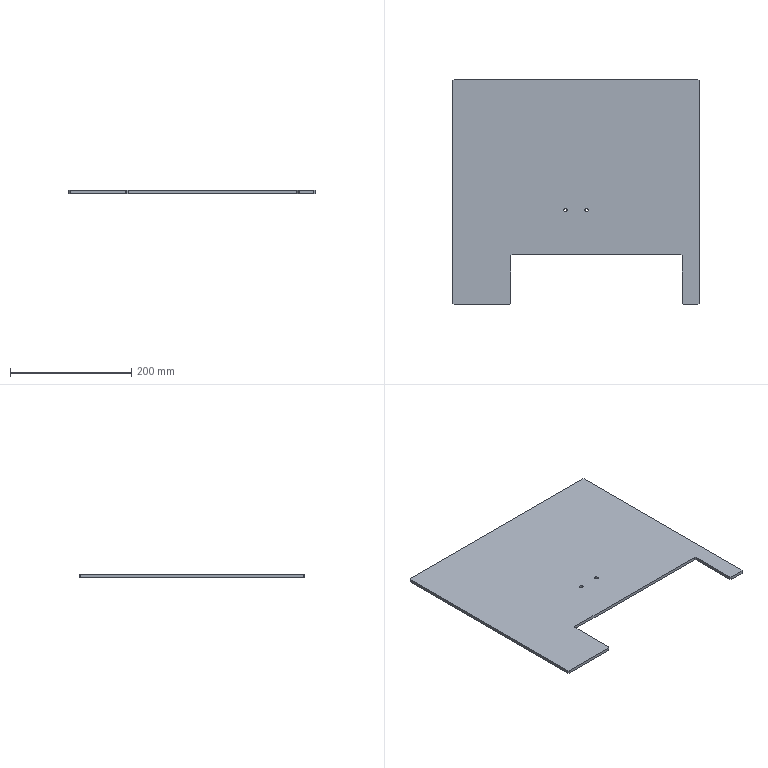Part | SolidWorks | features Extrusion 1, Fillet 1, HoleWzd 1, ICE 1 | 1 solid | 22 faces | box 406 x 372 x 5 mm | volume 637645 mm3 | plane 18 | cylinder 4 | commonest cylinder face diameters 5.5 x4
STEP:
#1=CARTESIAN_POINT('',(-20.25,-30.,0.));
#2=VERTEX_POINT('',#1);
#3=CARTESIAN_POINT('',(-14.75,-30.,0.));
#4=VERTEX_POINT('',#3);
#5=CARTESIAN_POINT('',(-17.5,-30.,0.));
#6=DIRECTION('',(0.,0.,1.));
#7=DIRECTION('',(1.,0.,0.));
#8=AXIS2_PLACEMENT_3D('',#5,#6,#7);
#9=CIRCLE('',#8,2.75);
#10=EDGE_CURVE('',#2,#4,#9,.T.);
#11=ORIENTED_EDGE('',*,*,#10,.F.);
#12=CARTESIAN_POINT('',(-20.25,-30.,5.));
#13=VERTEX_POINT('',#12);
#14=CARTESIAN_POINT('',(-20.25,-30.,5.));
#15=DIRECTION('',(0.,0.,1.));
#16=VECTOR('',#15,1000.);
#17=LINE('',#14,#16);
#18=EDGE_CURVE('',#2,#13,#17,.T.);
#19=ORIENTED_EDGE('',*,*,#18,.T.);
#20=CARTESIAN_POINT('',(-14.75,-30.,5.));
#21=VERTEX_POINT('',#20);
#22=CARTESIAN_POINT('',(-17.5,-30.,5.));
#23=DIRECTION('',(0.,0.,1.));
#24=DIRECTION('',(1.,0.,0.));
#25=AXIS2_PLACEMENT_3D('',#22,#23,#24);
#26=CIRCLE('',#25,2.75);
#27=EDGE_CURVE('',#13,#21,#26,.T.);
#28=ORIENTED_EDGE('',*,*,#27,.T.);
#29=CARTESIAN_POINT('',(-14.75,-30.,5.));
#30=DIRECTION('',(0.,0.,1.));
#31=VECTOR('',#30,1000.);
#32=LINE('',#29,#31);
#33=EDGE_CURVE('',#4,#21,#32,.T.);
#34=ORIENTED_EDGE('',*,*,#33,.F.);
#35=EDGE_LOOP('',(#11,#19,#28,#34));
#36=FACE_OUTER_BOUND('',#35,.T.);
#37=CARTESIAN_POINT('',(-17.5,-30.,5.));
#38=DIRECTION('',(0.,0.,1.));
#39=DIRECTION('',(1.,0.,0.));
#40=AXIS2_PLACEMENT_3D('',#37,#38,#39);
#41=CYLINDRICAL_SURFACE('',#40,2.75);
#42=ADVANCED_FACE('',(#36),#41,.F.);
#43=CARTESIAN_POINT('',(14.75,-30.,0.));
#44=VERTEX_POINT('',#43);
#45=CARTESIAN_POINT('',(20.25,-30.,0.));
#46=VERTEX_POINT('',#45);
#47=CARTESIAN_POINT('',(17.5,-30.,0.));
#48=DIRECTION('',(0.,0.,1.));
#49=DIRECTION('',(1.,0.,0.));
#50=AXIS2_PLACEMENT_3D('',#47,#48,#49);
#51=CIRCLE('',#50,2.75);
#52=EDGE_CURVE('',#44,#46,#51,.T.);
#53=ORIENTED_EDGE('',*,*,#52,.F.);
#54=CARTESIAN_POINT('',(14.75,-30.,5.));
#55=VERTEX_POINT('',#54);
#56=CARTESIAN_POINT('',(14.75,-30.,5.));
#57=DIRECTION('',(0.,0.,1.));
#58=VECTOR('',#57,1000.);
#59=LINE('',#56,#58);
#60=EDGE_CURVE('',#44,#55,#59,.T.);
#61=ORIENTED_EDGE('',*,*,#60,.T.);
#62=CARTESIAN_POINT('',(20.25,-30.,5.));
#63=VERTEX_POINT('',#62);
#64=CARTESIAN_POINT('',(17.5,-30.,5.));
#65=DIRECTION('',(0.,0.,1.));
#66=DIRECTION('',(1.,0.,0.));
#67=AXIS2_PLACEMENT_3D('',#64,#65,#66);
#68=CIRCLE('',#67,2.75);
#69=EDGE_CURVE('',#55,#63,#68,.T.);
#70=ORIENTED_EDGE('',*,*,#69,.T.);
#71=CARTESIAN_POINT('',(20.25,-30.,5.));
#72=DIRECTION('',(0.,0.,1.));
#73=VECTOR('',#72,1000.);
#74=LINE('',#71,#73);
#75=EDGE_CURVE('',#46,#63,#74,.T.);
#76=ORIENTED_EDGE('',*,*,#75,.F.);
#77=EDGE_LOOP('',(#53,#61,#70,#76));
#78=FACE_OUTER_BOUND('',#77,.T.);
#79=CARTESIAN_POINT('',(17.5,-30.,5.));
#80=DIRECTION('',(0.,0.,1.));
#81=DIRECTION('',(1.,0.,0.));
#82=AXIS2_PLACEMENT_3D('',#79,#80,#81);
#83=CYLINDRICAL_SURFACE('',#82,2.75);
#84=ADVANCED_FACE('',(#78),#83,.F.);
#85=CARTESIAN_POINT('',(-201.,-186.,0.));
#86=VERTEX_POINT('',#85);
#87=CARTESIAN_POINT('',(-109.5,-186.,0.));
#88=VERTEX_POINT('',#87);
#89=CARTESIAN_POINT('',(203.,-186.,0.));
#90=DIRECTION('',(1.,0.,0.));
#91=VECTOR('',#90,1000.);
#92=LINE('',#89,#91);
#93=EDGE_CURVE('',#86,#88,#92,.T.);
#94=ORIENTED_EDGE('',*,*,#93,.T.);
#95=CARTESIAN_POINT('',(-109.5,-186.,5.));
#96=VERTEX_POINT('',#95);
#97=CARTESIAN_POINT('',(-109.5,-186.,5.));
#98=DIRECTION('',(0.,0.,1.));
#99=VECTOR('',#98,1000.);
#100=LINE('',#97,#99);
#101=EDGE_CURVE('',#88,#96,#100,.T.);
#102=ORIENTED_EDGE('',*,*,#101,.T.);
#103=CARTESIAN_POINT('',(-201.,-186.,5.));
#104=VERTEX_POINT('',#103);
#105=CARTESIAN_POINT('',(203.,-186.,5.));
#106=DIRECTION('',(1.,0.,0.));
#107=VECTOR('',#106,1000.);
#108=LINE('',#105,#107);
#109=EDGE_CURVE('',#104,#96,#108,.T.);
#110=ORIENTED_EDGE('',*,*,#109,.F.);
#111=CARTESIAN_POINT('',(-201.,-186.,5.));
#112=DIRECTION('',(0.,0.,-1.));
#113=VECTOR('',#112,1000.);
#114=LINE('',#111,#113);
#115=EDGE_CURVE('',#104,#86,#114,.T.);
#116=ORIENTED_EDGE('',*,*,#115,.T.);
#117=EDGE_LOOP('',(#94,#102,#110,#116));
#118=FACE_OUTER_BOUND('',#117,.T.);
#119=CARTESIAN_POINT('',(203.,-186.,5.));
#120=DIRECTION('',(0.,1.,0.));
#121=DIRECTION('',(-1.,0.,0.));
#122=AXIS2_PLACEMENT_3D('',#119,#120,#121);
#123=PLANE('',#122);
#124=ADVANCED_FACE('',(#118),#123,.F.);
#125=CARTESIAN_POINT('',(-203.,184.,5.));
#126=VERTEX_POINT('',#125);
#127=CARTESIAN_POINT('',(-203.,-184.,5.));
#128=VERTEX_POINT('',#127);
#129=CARTESIAN_POINT('',(-203.,-186.,5.));
#130=DIRECTION('',(0.,-1.,0.));
#131=VECTOR('',#130,1000.);
#132=LINE('',#129,#131);
#133=EDGE_CURVE('',#126,#128,#132,.T.);
#134=ORIENTED_EDGE('',*,*,#133,.F.);
#135=CARTESIAN_POINT('',(-203.,184.,0.));
#136=VERTEX_POINT('',#135);
#137=CARTESIAN_POINT('',(-203.,184.,5.));
#138=DIRECTION('',(0.,0.,-1.));
#139=VECTOR('',#138,1000.);
#140=LINE('',#137,#139);
#141=EDGE_CURVE('',#126,#136,#140,.T.);
#142=ORIENTED_EDGE('',*,*,#141,.T.);
#143=CARTESIAN_POINT('',(-203.,-184.,0.));
#144=VERTEX_POINT('',#143);
#145=CARTESIAN_POINT('',(-203.,-186.,0.));
#146=DIRECTION('',(0.,-1.,0.));
#147=VECTOR('',#146,1000.);
#148=LINE('',#145,#147);
#149=EDGE_CURVE('',#136,#144,#148,.T.);
#150=ORIENTED_EDGE('',*,*,#149,.T.);
#151=CARTESIAN_POINT('',(-203.,-184.,5.));
#152=DIRECTION('',(0.,0.,1.));
#153=VECTOR('',#152,1000.);
#154=LINE('',#151,#153);
#155=EDGE_CURVE('',#144,#128,#154,.T.);
#156=ORIENTED_EDGE('',*,*,#155,.T.);
#157=EDGE_LOOP('',(#134,#142,#150,#156));
#158=FACE_OUTER_BOUND('',#157,.T.);
#159=CARTESIAN_POINT('',(-203.,-186.,5.));
#160=DIRECTION('',(1.,0.,0.));
#161=DIRECTION('',(0.,0.,-1.));
#162=AXIS2_PLACEMENT_3D('',#159,#160,#161);
#163=PLANE('',#162);
#164=ADVANCED_FACE('',(#158),#163,.F.);
#165=CARTESIAN_POINT('',(177.,-186.,5.));
#166=VERTEX_POINT('',#165);
#167=CARTESIAN_POINT('',(201.,-186.,5.));
#168=VERTEX_POINT('',#167);
#169=CARTESIAN_POINT('',(203.,-186.,5.));
#170=DIRECTION('',(1.,0.,0.));
#171=VECTOR('',#170,1000.);
#172=LINE('',#169,#171);
#173=EDGE_CURVE('',#166,#168,#172,.T.);
#174=ORIENTED_EDGE('',*,*,#173,.F.);
#175=CARTESIAN_POINT('',(177.,-186.,0.));
#176=VERTEX_POINT('',#175);
#177=CARTESIAN_POINT('',(177.,-186.,5.));
#178=DIRECTION('',(0.,0.,-1.));
#179=VECTOR('',#178,1000.);
#180=LINE('',#177,#179);
#181=EDGE_CURVE('',#166,#176,#180,.T.);
#182=ORIENTED_EDGE('',*,*,#181,.T.);
#183=CARTESIAN_POINT('',(201.,-186.,0.));
#184=VERTEX_POINT('',#183);
#185=CARTESIAN_POINT('',(203.,-186.,0.));
#186=DIRECTION('',(1.,0.,0.));
#187=VECTOR('',#186,1000.);
#188=LINE('',#185,#187);
#189=EDGE_CURVE('',#176,#184,#188,.T.);
#190=ORIENTED_EDGE('',*,*,#189,.T.);
#191=CARTESIAN_POINT('',(201.,-186.,5.));
#192=DIRECTION('',(0.,0.,1.));
#193=VECTOR('',#192,1000.);
#194=LINE('',#191,#193);
#195=EDGE_CURVE('',#184,#168,#194,.T.);
#196=ORIENTED_EDGE('',*,*,#195,.T.);
#197=EDGE_LOOP('',(#174,#182,#190,#196));
#198=FACE_OUTER_BOUND('',#197,.T.);
#199=CARTESIAN_POINT('',(203.,-186.,5.));
#200=DIRECTION('',(0.,1.,0.));
#201=DIRECTION('',(-1.,0.,0.));
#202=AXIS2_PLACEMENT_3D('',#199,#200,#201);
#203=PLANE('',#202);
#204=ADVANCED_FACE('',(#198),#203,.F.);
#205=CARTESIAN_POINT('',(203.,-184.,0.));
#206=VERTEX_POINT('',#205);
#207=CARTESIAN_POINT('',(203.,184.,0.));
#208=VERTEX_POINT('',#207);
#209=CARTESIAN_POINT('',(203.,-186.,0.));
#210=DIRECTION('',(0.,1.,0.));
#211=VECTOR('',#210,1000.);
#212=LINE('',#209,#211);
#213=EDGE_CURVE('',#206,#208,#212,.T.);
#214=ORIENTED_EDGE('',*,*,#213,.T.);
#215=CARTESIAN_POINT('',(203.,184.,5.));
#216=VERTEX_POINT('',#215);
#217=CARTESIAN_POINT('',(203.,184.,5.));
#218=DIRECTION('',(0.,0.,1.));
#219=VECTOR('',#218,1000.);
#220=LINE('',#217,#219);
#221=EDGE_CURVE('',#208,#216,#220,.T.);
#222=ORIENTED_EDGE('',*,*,#221,.T.);
#223=CARTESIAN_POINT('',(203.,-184.,5.));
#224=VERTEX_POINT('',#223);
#225=CARTESIAN_POINT('',(203.,-186.,5.));
#226=DIRECTION('',(0.,1.,0.));
#227=VECTOR('',#226,1000.);
#228=LINE('',#225,#227);
#229=EDGE_CURVE('',#224,#216,#228,.T.);
#230=ORIENTED_EDGE('',*,*,#229,.F.);
#231=CARTESIAN_POINT('',(203.,-184.,5.));
#232=DIRECTION('',(0.,0.,-1.));
#233=VECTOR('',#232,1000.);
#234=LINE('',#231,#233);
#235=EDGE_CURVE('',#224,#206,#234,.T.);
#236=ORIENTED_EDGE('',*,*,#235,.T.);
#237=EDGE_LOOP('',(#214,#222,#230,#236));
#238=FACE_OUTER_BOUND('',#237,.T.);
#239=CARTESIAN_POINT('',(203.,-186.,5.));
#240=DIRECTION('',(-1.,0.,0.));
#241=DIRECTION('',(0.,-1.,0.));
#242=AXIS2_PLACEMENT_3D('',#239,#240,#241);
#243=PLANE('',#242);
#244=ADVANCED_FACE('',(#238),#243,.F.);
#245=CARTESIAN_POINT('',(201.,186.,0.));
#246=VERTEX_POINT('',#245);
#247=CARTESIAN_POINT('',(-201.,186.,0.));
#248=VERTEX_POINT('',#247);
#249=CARTESIAN_POINT('',(203.,186.,0.));
#250=DIRECTION('',(-1.,0.,0.));
#251=VECTOR('',#250,1000.);
#252=LINE('',#249,#251);
#253=EDGE_CURVE('',#246,#248,#252,.T.);
#254=ORIENTED_EDGE('',*,*,#253,.T.);
#255=CARTESIAN_POINT('',(-201.,186.,5.));
#256=VERTEX_POINT('',#255);
#257=CARTESIAN_POINT('',(-201.,186.,5.));
#258=DIRECTION('',(0.,0.,1.));
#259=VECTOR('',#258,1000.);
#260=LINE('',#257,#259);
#261=EDGE_CURVE('',#248,#256,#260,.T.);
#262=ORIENTED_EDGE('',*,*,#261,.T.);
#263=CARTESIAN_POINT('',(201.,186.,5.));
#264=VERTEX_POINT('',#263);
#265=CARTESIAN_POINT('',(203.,186.,5.));
#266=DIRECTION('',(-1.,0.,0.));
#267=VECTOR('',#266,1000.);
#268=LINE('',#265,#267);
#269=EDGE_CURVE('',#264,#256,#268,.T.);
#270=ORIENTED_EDGE('',*,*,#269,.F.);
#271=CARTESIAN_POINT('',(201.,186.,5.));
#272=DIRECTION('',(0.,0.,-1.));
#273=VECTOR('',#272,1000.);
#274=LINE('',#271,#273);
#275=EDGE_CURVE('',#264,#246,#274,.T.);
#276=ORIENTED_EDGE('',*,*,#275,.T.);
#277=EDGE_LOOP('',(#254,#262,#270,#276));
#278=FACE_OUTER_BOUND('',#277,.T.);
#279=CARTESIAN_POINT('',(203.,186.,5.));
#280=DIRECTION('',(0.,-1.,0.));
#281=DIRECTION('',(1.,0.,0.));
#282=AXIS2_PLACEMENT_3D('',#279,#280,#281);
#283=PLANE('',#282);
#284=ADVANCED_FACE('',(#278),#283,.F.);
#285=CARTESIAN_POINT('',(-17.5,-30.,5.));
#286=DIRECTION('',(0.,0.,1.));
#287=DIRECTION('',(1.,0.,0.));
#288=AXIS2_PLACEMENT_3D('',#285,#286,#287);
#289=CIRCLE('',#288,2.75);
#290=EDGE_CURVE('',#21,#13,#289,.T.);
#291=ORIENTED_EDGE('',*,*,#290,.F.);
#292=ORIENTED_EDGE('',*,*,#27,.F.);
#293=EDGE_LOOP('',(#291,#292));
#294=FACE_BOUND('',#293,.T.);
#295=CARTESIAN_POINT('',(17.5,-30.,5.));
#296=DIRECTION('',(0.,0.,1.));
#297=DIRECTION('',(1.,0.,0.));
#298=AXIS2_PLACEMENT_3D('',#295,#296,#297);
#299=CIRCLE('',#298,2.75);
#300=EDGE_CURVE('',#63,#55,#299,.T.);
#301=ORIENTED_EDGE('',*,*,#300,.F.);
#302=ORIENTED_EDGE('',*,*,#69,.F.);
#303=EDGE_LOOP('',(#301,#302));
#304=FACE_BOUND('',#303,.T.);
#305=CARTESIAN_POINT('',(175.,-184.,5.));
#306=VERTEX_POINT('',#305);
#307=CARTESIAN_POINT('',(175.,-105.,5.));
#308=VERTEX_POINT('',#307);
#309=CARTESIAN_POINT('',(175.,-186.,5.));
#310=DIRECTION('',(0.,1.,0.));
#311=VECTOR('',#310,1000.);
#312=LINE('',#309,#311);
#313=EDGE_CURVE('',#306,#308,#312,.T.);
#314=ORIENTED_EDGE('',*,*,#313,.F.);
#315=CARTESIAN_POINT('',(-4.5,-4.5,5.));
#316=DIRECTION('',(0.7071,-0.7071,0.));
#317=VECTOR('',#316,1000.);
#318=LINE('',#315,#317);
#319=EDGE_CURVE('',#306,#166,#318,.T.);
#320=ORIENTED_EDGE('',*,*,#319,.T.);
#321=ORIENTED_EDGE('',*,*,#173,.T.);
#322=CARTESIAN_POINT('',(193.5,-193.5,5.));
#323=DIRECTION('',(0.7071,0.7071,0.));
#324=VECTOR('',#323,1000.);
#325=LINE('',#322,#324);
#326=EDGE_CURVE('',#168,#224,#325,.T.);
#327=ORIENTED_EDGE('',*,*,#326,.T.);
#328=ORIENTED_EDGE('',*,*,#229,.T.);
#329=CARTESIAN_POINT('',(193.5,193.5,5.));
#330=DIRECTION('',(-0.7071,0.7071,0.));
#331=VECTOR('',#330,1000.);
#332=LINE('',#329,#331);
#333=EDGE_CURVE('',#216,#264,#332,.T.);
#334=ORIENTED_EDGE('',*,*,#333,.T.);
#335=ORIENTED_EDGE('',*,*,#269,.T.);
#336=CARTESIAN_POINT('',(-193.5,193.5,5.));
#337=DIRECTION('',(-0.7071,-0.7071,0.));
#338=VECTOR('',#337,1000.);
#339=LINE('',#336,#338);
#340=EDGE_CURVE('',#256,#126,#339,.T.);
#341=ORIENTED_EDGE('',*,*,#340,.T.);
#342=ORIENTED_EDGE('',*,*,#133,.T.);
#343=CARTESIAN_POINT('',(-193.5,-193.5,5.));
#344=DIRECTION('',(0.7071,-0.7071,0.));
#345=VECTOR('',#344,1000.);
#346=LINE('',#343,#345);
#347=EDGE_CURVE('',#128,#104,#346,.T.);
#348=ORIENTED_EDGE('',*,*,#347,.T.);
#349=ORIENTED_EDGE('',*,*,#109,.T.);
#350=CARTESIAN_POINT('',(-107.5,-184.,5.));
#351=VERTEX_POINT('',#350);
#352=CARTESIAN_POINT('',(38.25,-38.25,5.));
#353=DIRECTION('',(0.7071,0.7071,0.));
#354=VECTOR('',#353,1000.);
#355=LINE('',#352,#354);
#356=EDGE_CURVE('',#96,#351,#355,.T.);
#357=ORIENTED_EDGE('',*,*,#356,.T.);
#358=CARTESIAN_POINT('',(-107.5,-105.,5.));
#359=VERTEX_POINT('',#358);
#360=CARTESIAN_POINT('',(-107.5,-186.,5.));
#361=DIRECTION('',(0.,-1.,0.));
#362=VECTOR('',#361,1000.);
#363=LINE('',#360,#362);
#364=EDGE_CURVE('',#359,#351,#363,.T.);
#365=ORIENTED_EDGE('',*,*,#364,.F.);
#366=CARTESIAN_POINT('',(-105.5,-103.,5.));
#367=VERTEX_POINT('',#366);
#368=CARTESIAN_POINT('',(-107.5,-105.,5.));
#369=DIRECTION('',(0.7071,0.7071,0.));
#370=VECTOR('',#369,1000.);
#371=LINE('',#368,#370);
#372=EDGE_CURVE('',#359,#367,#371,.T.);
#373=ORIENTED_EDGE('',*,*,#372,.T.);
#374=CARTESIAN_POINT('',(173.,-103.,5.));
#375=VERTEX_POINT('',#374);
#376=CARTESIAN_POINT('',(175.,-103.,5.));
#377=DIRECTION('',(-1.,0.,0.));
#378=VECTOR('',#377,1000.);
#379=LINE('',#376,#378);
#380=EDGE_CURVE('',#375,#367,#379,.T.);
#381=ORIENTED_EDGE('',*,*,#380,.F.);
#382=CARTESIAN_POINT('',(173.,-103.,5.));
#383=DIRECTION('',(0.7071,-0.7071,0.));
#384=VECTOR('',#383,1000.);
#385=LINE('',#382,#384);
#386=EDGE_CURVE('',#375,#308,#385,.T.);
#387=ORIENTED_EDGE('',*,*,#386,.T.);
#388=EDGE_LOOP('',(#314,#320,#321,#327,#328,#334,#335,#341,#342,#348,#349,#357,#365,#373,#381,#387));
#389=FACE_OUTER_BOUND('',#388,.T.);
#390=CARTESIAN_POINT('',(0.,0.,5.));
#391=DIRECTION('',(0.,0.,1.));
#392=DIRECTION('',(1.,0.,0.));
#393=AXIS2_PLACEMENT_3D('',#390,#391,#392);
#394=PLANE('',#393);
#395=ADVANCED_FACE('',(#294,#304,#389),#394,.T.);
#396=CARTESIAN_POINT('',(-17.5,-30.,0.));
#397=DIRECTION('',(0.,0.,1.));
#398=DIRECTION('',(1.,0.,0.));
#399=AXIS2_PLACEMENT_3D('',#396,#397,#398);
#400=CIRCLE('',#399,2.75);
#401=EDGE_CURVE('',#4,#2,#400,.T.);
#402=ORIENTED_EDGE('',*,*,#401,.T.);
#403=ORIENTED_EDGE('',*,*,#10,.T.);
#404=EDGE_LOOP('',(#402,#403));
#405=FACE_BOUND('',#404,.T.);
#406=CARTESIAN_POINT('',(17.5,-30.,0.));
#407=DIRECTION('',(0.,0.,1.));
#408=DIRECTION('',(1.,0.,0.));
#409=AXIS2_PLACEMENT_3D('',#406,#407,#408);
#410=CIRCLE('',#409,2.75);
#411=EDGE_CURVE('',#46,#44,#410,.T.);
#412=ORIENTED_EDGE('',*,*,#411,.T.);
#413=ORIENTED_EDGE('',*,*,#52,.T.);
#414=EDGE_LOOP('',(#412,#413));
#415=FACE_BOUND('',#414,.T.);
#416=ORIENTED_EDGE('',*,*,#189,.F.);
#417=CARTESIAN_POINT('',(175.,-184.,0.));
#418=VERTEX_POINT('',#417);
#419=CARTESIAN_POINT('',(175.,-184.,0.));
#420=DIRECTION('',(-0.7071,0.7071,0.));
#421=VECTOR('',#420,1000.);
#422=LINE('',#419,#421);
#423=EDGE_CURVE('',#176,#418,#422,.T.);
#424=ORIENTED_EDGE('',*,*,#423,.T.);
#425=CARTESIAN_POINT('',(175.,-105.,0.));
#426=VERTEX_POINT('',#425);
#427=CARTESIAN_POINT('',(175.,-186.,0.));
#428=DIRECTION('',(0.,1.,0.));
#429=VECTOR('',#428,1000.);
#430=LINE('',#427,#429);
#431=EDGE_CURVE('',#418,#426,#430,.T.);
#432=ORIENTED_EDGE('',*,*,#431,.T.);
#433=CARTESIAN_POINT('',(173.,-103.,0.));
#434=VERTEX_POINT('',#433);
#435=CARTESIAN_POINT('',(35.,35.,0.));
#436=DIRECTION('',(-0.7071,0.7071,0.));
#437=VECTOR('',#436,1000.);
#438=LINE('',#435,#437);
#439=EDGE_CURVE('',#426,#434,#438,.T.);
#440=ORIENTED_EDGE('',*,*,#439,.T.);
#441=CARTESIAN_POINT('',(-105.5,-103.,0.));
#442=VERTEX_POINT('',#441);
#443=CARTESIAN_POINT('',(175.,-103.,0.));
#444=DIRECTION('',(-1.,0.,0.));
#445=VECTOR('',#444,1000.);
#446=LINE('',#443,#445);
#447=EDGE_CURVE('',#434,#442,#446,.T.);
#448=ORIENTED_EDGE('',*,*,#447,.T.);
#449=CARTESIAN_POINT('',(-107.5,-105.,0.));
#450=VERTEX_POINT('',#449);
#451=CARTESIAN_POINT('',(-1.25,1.25,0.));
#452=DIRECTION('',(-0.7071,-0.7071,0.));
#453=VECTOR('',#452,1000.);
#454=LINE('',#451,#453);
#455=EDGE_CURVE('',#442,#450,#454,.T.);
#456=ORIENTED_EDGE('',*,*,#455,.T.);
#457=CARTESIAN_POINT('',(-107.5,-184.,0.));
#458=VERTEX_POINT('',#457);
#459=CARTESIAN_POINT('',(-107.5,-186.,0.));
#460=DIRECTION('',(0.,-1.,0.));
#461=VECTOR('',#460,1000.);
#462=LINE('',#459,#461);
#463=EDGE_CURVE('',#450,#458,#462,.T.);
#464=ORIENTED_EDGE('',*,*,#463,.T.);
#465=CARTESIAN_POINT('',(-109.5,-186.,0.));
#466=DIRECTION('',(-0.7071,-0.7071,0.));
#467=VECTOR('',#466,1000.);
#468=LINE('',#465,#467);
#469=EDGE_CURVE('',#458,#88,#468,.T.);
#470=ORIENTED_EDGE('',*,*,#469,.T.);
#471=ORIENTED_EDGE('',*,*,#93,.F.);
#472=CARTESIAN_POINT('',(-201.,-186.,0.));
#473=DIRECTION('',(-0.7071,0.7071,0.));
#474=VECTOR('',#473,1000.);
#475=LINE('',#472,#474);
#476=EDGE_CURVE('',#86,#144,#475,.T.);
#477=ORIENTED_EDGE('',*,*,#476,.T.);
#478=ORIENTED_EDGE('',*,*,#149,.F.);
#479=CARTESIAN_POINT('',(-203.,184.,0.));
#480=DIRECTION('',(0.7071,0.7071,0.));
#481=VECTOR('',#480,1000.);
#482=LINE('',#479,#481);
#483=EDGE_CURVE('',#136,#248,#482,.T.);
#484=ORIENTED_EDGE('',*,*,#483,.T.);
#485=ORIENTED_EDGE('',*,*,#253,.F.);
#486=CARTESIAN_POINT('',(201.,186.,0.));
#487=DIRECTION('',(0.7071,-0.7071,0.));
#488=VECTOR('',#487,1000.);
#489=LINE('',#486,#488);
#490=EDGE_CURVE('',#246,#208,#489,.T.);
#491=ORIENTED_EDGE('',*,*,#490,.T.);
#492=ORIENTED_EDGE('',*,*,#213,.F.);
#493=CARTESIAN_POINT('',(203.,-184.,0.));
#494=DIRECTION('',(-0.7071,-0.7071,0.));
#495=VECTOR('',#494,1000.);
#496=LINE('',#493,#495);
#497=EDGE_CURVE('',#206,#184,#496,.T.);
#498=ORIENTED_EDGE('',*,*,#497,.T.);
#499=EDGE_LOOP('',(#416,#424,#432,#440,#448,#456,#464,#470,#471,#477,#478,#484,#485,#491,#492,#498));
#500=FACE_OUTER_BOUND('',#499,.T.);
#501=CARTESIAN_POINT('',(0.,0.,0.));
#502=DIRECTION('',(0.,0.,1.));
#503=DIRECTION('',(1.,0.,0.));
#504=AXIS2_PLACEMENT_3D('',#501,#502,#503);
#505=PLANE('',#504);
#506=ADVANCED_FACE('',(#405,#415,#500),#505,.F.);
#507=ORIENTED_EDGE('',*,*,#364,.T.);
#508=CARTESIAN_POINT('',(-107.5,-184.,0.));
#509=DIRECTION('',(0.,0.,-1.));
#510=VECTOR('',#509,1000.);
#511=LINE('',#508,#510);
#512=EDGE_CURVE('',#351,#458,#511,.T.);
#513=ORIENTED_EDGE('',*,*,#512,.T.);
#514=ORIENTED_EDGE('',*,*,#463,.F.);
#515=CARTESIAN_POINT('',(-107.5,-105.,5.));
#516=DIRECTION('',(0.,0.,1.));
#517=VECTOR('',#516,1000.);
#518=LINE('',#515,#517);
#519=EDGE_CURVE('',#450,#359,#518,.T.);
#520=ORIENTED_EDGE('',*,*,#519,.T.);
#521=EDGE_LOOP('',(#507,#513,#514,#520));
#522=FACE_OUTER_BOUND('',#521,.T.);
#523=CARTESIAN_POINT('',(-107.5,-186.,0.));
#524=DIRECTION('',(-1.,0.,0.));
#525=DIRECTION('',(0.,-1.,0.));
#526=AXIS2_PLACEMENT_3D('',#523,#524,#525);
#527=PLANE('',#526);
#528=ADVANCED_FACE('',(#522),#527,.F.);
#529=ORIENTED_EDGE('',*,*,#447,.F.);
#530=CARTESIAN_POINT('',(173.,-103.,5.));
#531=DIRECTION('',(0.,0.,1.));
#532=VECTOR('',#531,1000.);
#533=LINE('',#530,#532);
#534=EDGE_CURVE('',#434,#375,#533,.T.);
#535=ORIENTED_EDGE('',*,*,#534,.T.);
#536=ORIENTED_EDGE('',*,*,#380,.T.);
#537=CARTESIAN_POINT('',(-105.5,-103.,0.));
#538=DIRECTION('',(0.,0.,-1.));
#539=VECTOR('',#538,1000.);
#540=LINE('',#537,#539);
#541=EDGE_CURVE('',#367,#442,#540,.T.);
#542=ORIENTED_EDGE('',*,*,#541,.T.);
#543=EDGE_LOOP('',(#529,#535,#536,#542));
#544=FACE_OUTER_BOUND('',#543,.T.);
#545=CARTESIAN_POINT('',(175.,-103.,0.));
#546=DIRECTION('',(0.,1.,0.));
#547=DIRECTION('',(-1.,0.,0.));
#548=AXIS2_PLACEMENT_3D('',#545,#546,#547);
#549=PLANE('',#548);
#550=ADVANCED_FACE('',(#544),#549,.F.);
#551=ORIENTED_EDGE('',*,*,#431,.F.);
#552=CARTESIAN_POINT('',(175.,-184.,0.));
#553=DIRECTION('',(0.,0.,1.));
#554=VECTOR('',#553,1000.);
#555=LINE('',#552,#554);
#556=EDGE_CURVE('',#418,#306,#555,.T.);
#557=ORIENTED_EDGE('',*,*,#556,.T.);
#558=ORIENTED_EDGE('',*,*,#313,.T.);
#559=CARTESIAN_POINT('',(175.,-105.,0.));
#560=DIRECTION('',(0.,0.,-1.));
#561=VECTOR('',#560,1000.);
#562=LINE('',#559,#561);
#563=EDGE_CURVE('',#308,#426,#562,.T.);
#564=ORIENTED_EDGE('',*,*,#563,.T.);
#565=EDGE_LOOP('',(#551,#557,#558,#564));
#566=FACE_OUTER_BOUND('',#565,.T.);
#567=CARTESIAN_POINT('',(175.,-186.,0.));
#568=DIRECTION('',(1.,0.,0.));
#569=DIRECTION('',(0.,0.,-1.));
#570=AXIS2_PLACEMENT_3D('',#567,#568,#569);
#571=PLANE('',#570);
#572=ADVANCED_FACE('',(#566),#571,.F.);
#573=ORIENTED_EDGE('',*,*,#60,.F.);
#574=ORIENTED_EDGE('',*,*,#411,.F.);
#575=ORIENTED_EDGE('',*,*,#75,.T.);
#576=ORIENTED_EDGE('',*,*,#300,.T.);
#577=EDGE_LOOP('',(#573,#574,#575,#576));
#578=FACE_OUTER_BOUND('',#577,.T.);
#579=CARTESIAN_POINT('',(17.5,-30.,5.));
#580=DIRECTION('',(0.,0.,1.));
#581=DIRECTION('',(1.,0.,0.));
#582=AXIS2_PLACEMENT_3D('',#579,#580,#581);
#583=CYLINDRICAL_SURFACE('',#582,2.75);
#584=ADVANCED_FACE('',(#578),#583,.F.);
#585=ORIENTED_EDGE('',*,*,#18,.F.);
#586=ORIENTED_EDGE('',*,*,#401,.F.);
#587=ORIENTED_EDGE('',*,*,#33,.T.);
#588=ORIENTED_EDGE('',*,*,#290,.T.);
#589=EDGE_LOOP('',(#585,#586,#587,#588));
#590=FACE_OUTER_BOUND('',#589,.T.);
#591=CARTESIAN_POINT('',(-17.5,-30.,5.));
#592=DIRECTION('',(0.,0.,1.));
#593=DIRECTION('',(1.,0.,0.));
#594=AXIS2_PLACEMENT_3D('',#591,#592,#593);
#595=CYLINDRICAL_SURFACE('',#594,2.75);
#596=ADVANCED_FACE('',(#590),#595,.F.);
#597=ORIENTED_EDGE('',*,*,#423,.F.);
#598=ORIENTED_EDGE('',*,*,#181,.F.);
#599=ORIENTED_EDGE('',*,*,#319,.F.);
#600=ORIENTED_EDGE('',*,*,#556,.F.);
#601=EDGE_LOOP('',(#597,#598,#599,#600));
#602=FACE_OUTER_BOUND('',#601,.T.);
#603=CARTESIAN_POINT('',(175.,-184.,0.));
#604=DIRECTION('',(0.7071,0.7071,0.));
#605=DIRECTION('',(0.,0.,1.));
#606=AXIS2_PLACEMENT_3D('',#603,#604,#605);
#607=PLANE('',#606);
#608=ADVANCED_FACE('',(#602),#607,.F.);
#609=ORIENTED_EDGE('',*,*,#469,.F.);
#610=ORIENTED_EDGE('',*,*,#512,.F.);
#611=ORIENTED_EDGE('',*,*,#356,.F.);
#612=ORIENTED_EDGE('',*,*,#101,.F.);
#613=EDGE_LOOP('',(#609,#610,#611,#612));
#614=FACE_OUTER_BOUND('',#613,.T.);
#615=CARTESIAN_POINT('',(-109.5,-186.,5.));
#616=DIRECTION('',(-0.7071,0.7071,0.));
#617=DIRECTION('',(0.,0.,1.));
#618=AXIS2_PLACEMENT_3D('',#615,#616,#617);
#619=PLANE('',#618);
#620=ADVANCED_FACE('',(#614),#619,.F.);
#621=ORIENTED_EDGE('',*,*,#340,.F.);
#622=ORIENTED_EDGE('',*,*,#261,.F.);
#623=ORIENTED_EDGE('',*,*,#483,.F.);
#624=ORIENTED_EDGE('',*,*,#141,.F.);
#625=EDGE_LOOP('',(#621,#622,#623,#624));
#626=FACE_OUTER_BOUND('',#625,.T.);
#627=CARTESIAN_POINT('',(-203.,184.,5.));
#628=DIRECTION('',(0.7071,-0.7071,0.));
#629=DIRECTION('',(0.,0.,-1.));
#630=AXIS2_PLACEMENT_3D('',#627,#628,#629);
#631=PLANE('',#630);
#632=ADVANCED_FACE('',(#626),#631,.F.);
#633=ORIENTED_EDGE('',*,*,#333,.F.);
#634=ORIENTED_EDGE('',*,*,#221,.F.);
#635=ORIENTED_EDGE('',*,*,#490,.F.);
#636=ORIENTED_EDGE('',*,*,#275,.F.);
#637=EDGE_LOOP('',(#633,#634,#635,#636));
#638=FACE_OUTER_BOUND('',#637,.T.);
#639=CARTESIAN_POINT('',(201.,186.,5.));
#640=DIRECTION('',(-0.7071,-0.7071,0.));
#641=DIRECTION('',(0.,0.,-1.));
#642=AXIS2_PLACEMENT_3D('',#639,#640,#641);
#643=PLANE('',#642);
#644=ADVANCED_FACE('',(#638),#643,.F.);
#645=ORIENTED_EDGE('',*,*,#326,.F.);
#646=ORIENTED_EDGE('',*,*,#195,.F.);
#647=ORIENTED_EDGE('',*,*,#497,.F.);
#648=ORIENTED_EDGE('',*,*,#235,.F.);
#649=EDGE_LOOP('',(#645,#646,#647,#648));
#650=FACE_OUTER_BOUND('',#649,.T.);
#651=CARTESIAN_POINT('',(203.,-184.,5.));
#652=DIRECTION('',(-0.7071,0.7071,0.));
#653=DIRECTION('',(0.,0.,-1.));
#654=AXIS2_PLACEMENT_3D('',#651,#652,#653);
#655=PLANE('',#654);
#656=ADVANCED_FACE('',(#650),#655,.F.);
#657=ORIENTED_EDGE('',*,*,#347,.F.);
#658=ORIENTED_EDGE('',*,*,#155,.F.);
#659=ORIENTED_EDGE('',*,*,#476,.F.);
#660=ORIENTED_EDGE('',*,*,#115,.F.);
#661=EDGE_LOOP('',(#657,#658,#659,#660));
#662=FACE_OUTER_BOUND('',#661,.T.);
#663=CARTESIAN_POINT('',(-201.,-186.,5.));
#664=DIRECTION('',(0.7071,0.7071,0.));
#665=DIRECTION('',(0.,0.,-1.));
#666=AXIS2_PLACEMENT_3D('',#663,#664,#665);
#667=PLANE('',#666);
#668=ADVANCED_FACE('',(#662),#667,.F.);
#669=ORIENTED_EDGE('',*,*,#439,.F.);
#670=ORIENTED_EDGE('',*,*,#563,.F.);
#671=ORIENTED_EDGE('',*,*,#386,.F.);
#672=ORIENTED_EDGE('',*,*,#534,.F.);
#673=EDGE_LOOP('',(#669,#670,#671,#672));
#674=FACE_OUTER_BOUND('',#673,.T.);
#675=CARTESIAN_POINT('',(173.,-103.,0.));
#676=DIRECTION('',(-0.7071,-0.7071,0.));
#677=DIRECTION('',(0.,0.,-1.));
#678=AXIS2_PLACEMENT_3D('',#675,#676,#677);
#679=PLANE('',#678);
#680=ADVANCED_FACE('',(#674),#679,.T.);
#681=ORIENTED_EDGE('',*,*,#455,.F.);
#682=ORIENTED_EDGE('',*,*,#541,.F.);
#683=ORIENTED_EDGE('',*,*,#372,.F.);
#684=ORIENTED_EDGE('',*,*,#519,.F.);
#685=EDGE_LOOP('',(#681,#682,#683,#684));
#686=FACE_OUTER_BOUND('',#685,.T.);
#687=CARTESIAN_POINT('',(-107.5,-105.,0.));
#688=DIRECTION('',(0.7071,-0.7071,0.));
#689=DIRECTION('',(0.,0.,-1.));
#690=AXIS2_PLACEMENT_3D('',#687,#688,#689);
#691=PLANE('',#690);
#692=ADVANCED_FACE('',(#686),#691,.T.);
#693=CLOSED_SHELL('',(#42,#84,#124,#164,#204,#244,#284,#395,#506,#528,#550,#572,#584,#596,#608,#620,#632,#644,#656,#668,#680,#692));
#694=MANIFOLD_SOLID_BREP('',#693);
#695=CARTESIAN_POINT('',(0.,0.,0.));
#696=DIRECTION('',(0.,0.,1.));
#697=DIRECTION('',(1.,0.,0.));
#698=AXIS2_PLACEMENT_3D('',#695,#696,#697);
#699=(LENGTH_UNIT()NAMED_UNIT(*)SI_UNIT(.MILLI.,.METRE.));
#700=UNCERTAINTY_MEASURE_WITH_UNIT(LENGTH_MEASURE(0.00001),#699,'','');
#701=(NAMED_UNIT(*)PLANE_ANGLE_UNIT()SI_UNIT($,.RADIAN.));
#702=(NAMED_UNIT(*)SI_UNIT($,.STERADIAN.)SOLID_ANGLE_UNIT());
#703=(GEOMETRIC_REPRESENTATION_CONTEXT(3)GLOBAL_UNCERTAINTY_ASSIGNED_CONTEXT((#700))GLOBAL_UNIT_ASSIGNED_CONTEXT((#699,#701,#702))REPRESENTATION_CONTEXT('',''));
#704=ADVANCED_BREP_SHAPE_REPRESENTATION('',(#694,#698),#703);